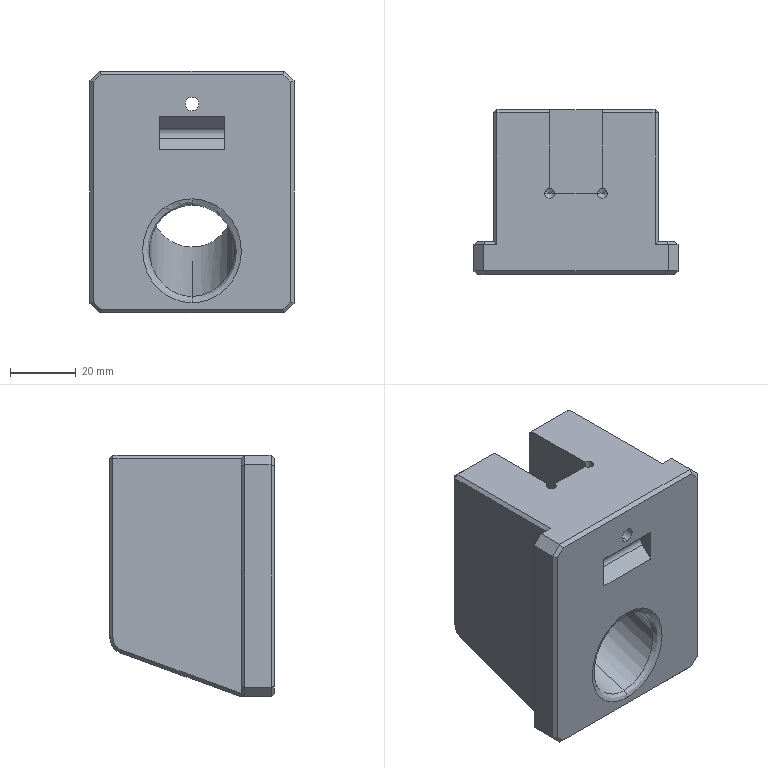Part | STEP file | Gaveta - Torre - 1 cav | 1 solid | 71 faces | box 62 x 50 x 73.5 mm | volume 139216 mm3 | plane 51 | cylinder 10 | cone 6 | spline 4 | commonest cylinder face diameters 3 x4 4.2 x2 26 x2 4 x1 10 x1